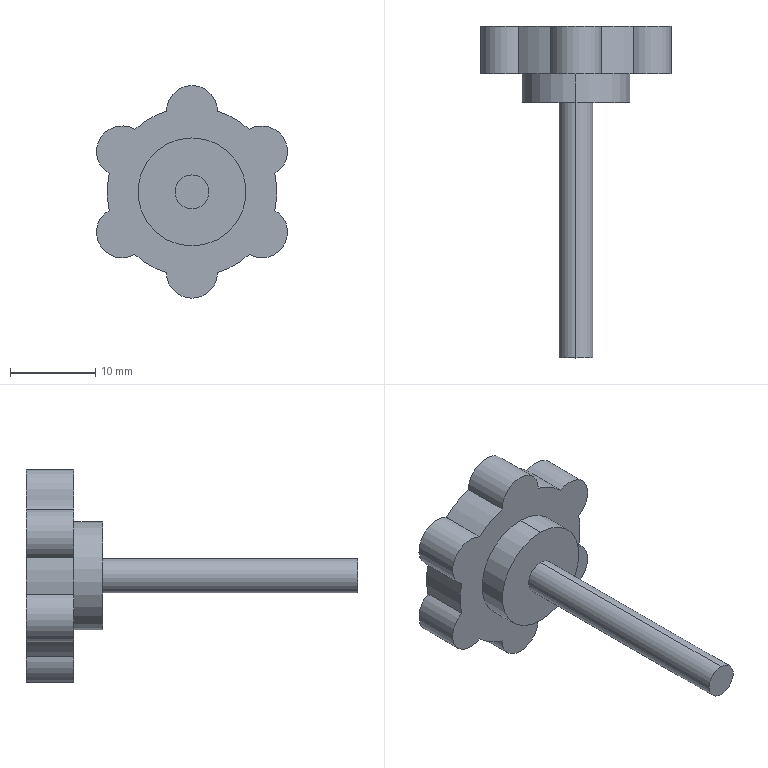Part | SolidWorks | features ICE 2, Extrusion 1 | 1 solid | 34 faces | box 22.455 x 39 x 25 mm | volume 2966 mm3 | cylinder 19 | plane 15 | commonest cylinder face diameters 6 x9 19.922 x6 4 x2 12.7 x2
STEP:
#1=CARTESIAN_POINT('',(0.,-33.4,-2.));
#2=VERTEX_POINT('',#1);
#3=CARTESIAN_POINT('',(0.,-33.4,2.));
#4=VERTEX_POINT('',#3);
#5=CARTESIAN_POINT('',(0.,-33.4,0.));
#6=DIRECTION('',(0.,-1.,0.));
#7=DIRECTION('',(0.,0.,-1.));
#8=AXIS2_PLACEMENT_3D('',#5,#6,#7);
#9=CIRCLE('',#8,2.);
#10=EDGE_CURVE('',#2,#4,#9,.T.);
#11=ORIENTED_EDGE('',*,*,#10,.F.);
#12=CARTESIAN_POINT('',(0.,-3.4,-2.));
#13=VERTEX_POINT('',#12);
#14=CARTESIAN_POINT('',(0.,-33.4,-2.));
#15=DIRECTION('',(0.,1.,0.));
#16=VECTOR('',#15,1000.);
#17=LINE('',#14,#16);
#18=EDGE_CURVE('',#2,#13,#17,.T.);
#19=ORIENTED_EDGE('',*,*,#18,.T.);
#20=CARTESIAN_POINT('',(0.,-3.4,2.));
#21=VERTEX_POINT('',#20);
#22=CARTESIAN_POINT('',(0.,-3.4,0.));
#23=DIRECTION('',(0.,-1.,0.));
#24=DIRECTION('',(0.,0.,-1.));
#25=AXIS2_PLACEMENT_3D('',#22,#23,#24);
#26=CIRCLE('',#25,2.);
#27=EDGE_CURVE('',#13,#21,#26,.T.);
#28=ORIENTED_EDGE('',*,*,#27,.T.);
#29=CARTESIAN_POINT('',(0.,-33.4,2.));
#30=DIRECTION('',(0.,1.,0.));
#31=VECTOR('',#30,1000.);
#32=LINE('',#29,#31);
#33=EDGE_CURVE('',#4,#21,#32,.T.);
#34=ORIENTED_EDGE('',*,*,#33,.F.);
#35=EDGE_LOOP('',(#11,#19,#28,#34));
#36=FACE_OUTER_BOUND('',#35,.T.);
#37=CARTESIAN_POINT('',(0.,-33.4,0.));
#38=DIRECTION('',(0.,1.,0.));
#39=DIRECTION('',(0.,0.,1.));
#40=AXIS2_PLACEMENT_3D('',#37,#38,#39);
#41=CYLINDRICAL_SURFACE('',#40,2.);
#42=ADVANCED_FACE('',(#36),#41,.T.);
#43=CARTESIAN_POINT('',(0.,-3.4,-6.35));
#44=VERTEX_POINT('',#43);
#45=CARTESIAN_POINT('',(0.,-3.4,6.35));
#46=VERTEX_POINT('',#45);
#47=CARTESIAN_POINT('',(0.,-3.4,0.));
#48=DIRECTION('',(0.,-1.,0.));
#49=DIRECTION('',(0.,0.,-1.));
#50=AXIS2_PLACEMENT_3D('',#47,#48,#49);
#51=CIRCLE('',#50,6.35);
#52=EDGE_CURVE('',#44,#46,#51,.T.);
#53=ORIENTED_EDGE('',*,*,#52,.F.);
#54=CARTESIAN_POINT('',(0.,0.,-6.35));
#55=VERTEX_POINT('',#54);
#56=CARTESIAN_POINT('',(0.,-3.4,-6.35));
#57=DIRECTION('',(0.,1.,0.));
#58=VECTOR('',#57,1000.);
#59=LINE('',#56,#58);
#60=EDGE_CURVE('',#44,#55,#59,.T.);
#61=ORIENTED_EDGE('',*,*,#60,.T.);
#62=CARTESIAN_POINT('',(0.,0.,6.35));
#63=VERTEX_POINT('',#62);
#64=CARTESIAN_POINT('',(0.,0.,0.));
#65=DIRECTION('',(0.,-1.,0.));
#66=DIRECTION('',(0.,0.,1.));
#67=AXIS2_PLACEMENT_3D('',#64,#65,#66);
#68=CIRCLE('',#67,6.35);
#69=EDGE_CURVE('',#55,#63,#68,.T.);
#70=ORIENTED_EDGE('',*,*,#69,.T.);
#71=CARTESIAN_POINT('',(0.,-3.4,6.35));
#72=DIRECTION('',(0.,1.,0.));
#73=VECTOR('',#72,1000.);
#74=LINE('',#71,#73);
#75=EDGE_CURVE('',#46,#63,#74,.T.);
#76=ORIENTED_EDGE('',*,*,#75,.F.);
#77=EDGE_LOOP('',(#53,#61,#70,#76));
#78=FACE_OUTER_BOUND('',#77,.T.);
#79=CARTESIAN_POINT('',(0.,-3.4,0.));
#80=DIRECTION('',(0.,1.,0.));
#81=DIRECTION('',(0.,0.,1.));
#82=AXIS2_PLACEMENT_3D('',#79,#80,#81);
#83=CYLINDRICAL_SURFACE('',#82,6.35);
#84=ADVANCED_FACE('',(#78),#83,.T.);
#85=CARTESIAN_POINT('',(8.228,5.6,-7.751));
#86=VERTEX_POINT('',#85);
#87=CARTESIAN_POINT('',(6.728,5.6,-7.349));
#88=VERTEX_POINT('',#87);
#89=CARTESIAN_POINT('',(8.228,5.6,-4.751));
#90=DIRECTION('',(0.,1.,0.));
#91=DIRECTION('',(0.,0.,1.));
#92=AXIS2_PLACEMENT_3D('',#89,#90,#91);
#93=CIRCLE('',#92,3.);
#94=EDGE_CURVE('',#86,#88,#93,.T.);
#95=ORIENTED_EDGE('',*,*,#94,.F.);
#96=CARTESIAN_POINT('',(8.228,0.,-7.751));
#97=VERTEX_POINT('',#96);
#98=CARTESIAN_POINT('',(8.228,5.6,-7.751));
#99=DIRECTION('',(0.,-1.,0.));
#100=VECTOR('',#99,1000.);
#101=LINE('',#98,#100);
#102=EDGE_CURVE('',#86,#97,#101,.T.);
#103=ORIENTED_EDGE('',*,*,#102,.T.);
#104=CARTESIAN_POINT('',(6.728,0.,-7.349));
#105=VERTEX_POINT('',#104);
#106=CARTESIAN_POINT('',(8.228,0.,-4.751));
#107=DIRECTION('',(0.,1.,0.));
#108=DIRECTION('',(0.,0.,1.));
#109=AXIS2_PLACEMENT_3D('',#106,#107,#108);
#110=CIRCLE('',#109,3.);
#111=EDGE_CURVE('',#97,#105,#110,.T.);
#112=ORIENTED_EDGE('',*,*,#111,.T.);
#113=CARTESIAN_POINT('',(6.728,5.6,-7.349));
#114=DIRECTION('',(0.,-1.,0.));
#115=VECTOR('',#114,1000.);
#116=LINE('',#113,#115);
#117=EDGE_CURVE('',#88,#105,#116,.T.);
#118=ORIENTED_EDGE('',*,*,#117,.F.);
#119=EDGE_LOOP('',(#95,#103,#112,#118));
#120=FACE_OUTER_BOUND('',#119,.T.);
#121=CARTESIAN_POINT('',(8.228,5.6,-4.751));
#122=DIRECTION('',(0.,-1.,0.));
#123=DIRECTION('',(0.,0.,-1.));
#124=AXIS2_PLACEMENT_3D('',#121,#122,#123);
#125=CYLINDRICAL_SURFACE('',#124,3.);
#126=ADVANCED_FACE('',(#120),#125,.T.);
#127=CARTESIAN_POINT('',(-8.227,5.6,-7.749));
#128=VERTEX_POINT('',#127);
#129=CARTESIAN_POINT('',(-9.727,5.6,-2.151));
#130=VERTEX_POINT('',#129);
#131=CARTESIAN_POINT('',(-8.227,5.6,-4.749));
#132=DIRECTION('',(0.,1.,0.));
#133=DIRECTION('',(0.,0.,1.));
#134=AXIS2_PLACEMENT_3D('',#131,#132,#133);
#135=CIRCLE('',#134,3.);
#136=EDGE_CURVE('',#128,#130,#135,.T.);
#137=ORIENTED_EDGE('',*,*,#136,.F.);
#138=CARTESIAN_POINT('',(-8.227,0.,-7.749));
#139=VERTEX_POINT('',#138);
#140=CARTESIAN_POINT('',(-8.227,5.6,-7.749));
#141=DIRECTION('',(0.,-1.,0.));
#142=VECTOR('',#141,1000.);
#143=LINE('',#140,#142);
#144=EDGE_CURVE('',#128,#139,#143,.T.);
#145=ORIENTED_EDGE('',*,*,#144,.T.);
#146=CARTESIAN_POINT('',(-9.727,0.,-2.151));
#147=VERTEX_POINT('',#146);
#148=CARTESIAN_POINT('',(-8.227,0.,-4.749));
#149=DIRECTION('',(0.,1.,0.));
#150=DIRECTION('',(0.,0.,1.));
#151=AXIS2_PLACEMENT_3D('',#148,#149,#150);
#152=CIRCLE('',#151,3.);
#153=EDGE_CURVE('',#139,#147,#152,.T.);
#154=ORIENTED_EDGE('',*,*,#153,.T.);
#155=CARTESIAN_POINT('',(-9.727,5.6,-2.151));
#156=DIRECTION('',(0.,-1.,0.));
#157=VECTOR('',#156,1000.);
#158=LINE('',#155,#157);
#159=EDGE_CURVE('',#130,#147,#158,.T.);
#160=ORIENTED_EDGE('',*,*,#159,.F.);
#161=EDGE_LOOP('',(#137,#145,#154,#160));
#162=FACE_OUTER_BOUND('',#161,.T.);
#163=CARTESIAN_POINT('',(-8.227,5.6,-4.749));
#164=DIRECTION('',(0.,-1.,0.));
#165=DIRECTION('',(0.,0.,-1.));
#166=AXIS2_PLACEMENT_3D('',#163,#164,#165);
#167=CYLINDRICAL_SURFACE('',#166,3.);
#168=ADVANCED_FACE('',(#162),#167,.T.);
#169=CARTESIAN_POINT('',(0.,5.6,-12.5));
#170=VERTEX_POINT('',#169);
#171=CARTESIAN_POINT('',(-3.,5.6,-9.5));
#172=VERTEX_POINT('',#171);
#173=CARTESIAN_POINT('',(0.,5.6,-9.5));
#174=DIRECTION('',(0.,1.,0.));
#175=DIRECTION('',(0.,0.,1.));
#176=AXIS2_PLACEMENT_3D('',#173,#174,#175);
#177=CIRCLE('',#176,3.);
#178=EDGE_CURVE('',#170,#172,#177,.T.);
#179=ORIENTED_EDGE('',*,*,#178,.F.);
#180=CARTESIAN_POINT('',(0.,0.,-12.5));
#181=VERTEX_POINT('',#180);
#182=CARTESIAN_POINT('',(0.,5.6,-12.5));
#183=DIRECTION('',(0.,-1.,0.));
#184=VECTOR('',#183,1000.);
#185=LINE('',#182,#184);
#186=EDGE_CURVE('',#170,#181,#185,.T.);
#187=ORIENTED_EDGE('',*,*,#186,.T.);
#188=CARTESIAN_POINT('',(-3.,0.,-9.5));
#189=VERTEX_POINT('',#188);
#190=CARTESIAN_POINT('',(0.,0.,-9.5));
#191=DIRECTION('',(0.,1.,0.));
#192=DIRECTION('',(0.,0.,1.));
#193=AXIS2_PLACEMENT_3D('',#190,#191,#192);
#194=CIRCLE('',#193,3.);
#195=EDGE_CURVE('',#181,#189,#194,.T.);
#196=ORIENTED_EDGE('',*,*,#195,.T.);
#197=CARTESIAN_POINT('',(-3.,5.6,-9.5));
#198=DIRECTION('',(0.,-1.,0.));
#199=VECTOR('',#198,1000.);
#200=LINE('',#197,#199);
#201=EDGE_CURVE('',#172,#189,#200,.T.);
#202=ORIENTED_EDGE('',*,*,#201,.F.);
#203=EDGE_LOOP('',(#179,#187,#196,#202));
#204=FACE_OUTER_BOUND('',#203,.T.);
#205=CARTESIAN_POINT('',(0.,5.6,-9.5));
#206=DIRECTION('',(0.,-1.,0.));
#207=DIRECTION('',(0.,0.,-1.));
#208=AXIS2_PLACEMENT_3D('',#205,#206,#207);
#209=CYLINDRICAL_SURFACE('',#208,3.);
#210=ADVANCED_FACE('',(#204),#209,.T.);
#211=ORIENTED_EDGE('',*,*,#186,.F.);
#212=CARTESIAN_POINT('',(3.,5.6,-9.5));
#213=VERTEX_POINT('',#212);
#214=CARTESIAN_POINT('',(0.,5.6,-9.5));
#215=DIRECTION('',(0.,1.,0.));
#216=DIRECTION('',(0.,0.,1.));
#217=AXIS2_PLACEMENT_3D('',#214,#215,#216);
#218=CIRCLE('',#217,3.);
#219=EDGE_CURVE('',#213,#170,#218,.T.);
#220=ORIENTED_EDGE('',*,*,#219,.F.);
#221=CARTESIAN_POINT('',(3.,0.,-9.5));
#222=VERTEX_POINT('',#221);
#223=CARTESIAN_POINT('',(3.,5.6,-9.5));
#224=DIRECTION('',(0.,-1.,0.));
#225=VECTOR('',#224,1000.);
#226=LINE('',#223,#225);
#227=EDGE_CURVE('',#213,#222,#226,.T.);
#228=ORIENTED_EDGE('',*,*,#227,.T.);
#229=CARTESIAN_POINT('',(0.,0.,-9.5));
#230=DIRECTION('',(0.,1.,0.));
#231=DIRECTION('',(0.,0.,1.));
#232=AXIS2_PLACEMENT_3D('',#229,#230,#231);
#233=CIRCLE('',#232,3.);
#234=EDGE_CURVE('',#222,#181,#233,.T.);
#235=ORIENTED_EDGE('',*,*,#234,.T.);
#236=EDGE_LOOP('',(#211,#220,#228,#235));
#237=FACE_OUTER_BOUND('',#236,.T.);
#238=CARTESIAN_POINT('',(0.,5.6,-9.5));
#239=DIRECTION('',(0.,-1.,0.));
#240=DIRECTION('',(0.,0.,-1.));
#241=AXIS2_PLACEMENT_3D('',#238,#239,#240);
#242=CYLINDRICAL_SURFACE('',#241,3.);
#243=ADVANCED_FACE('',(#237),#242,.T.);
#244=CARTESIAN_POINT('',(-3.,0.,-9.499));
#245=VERTEX_POINT('',#244);
#246=CARTESIAN_POINT('',(-3.,0.,-9.499));
#247=DIRECTION('',(0.,0.,1.));
#248=VECTOR('',#247,1000.);
#249=LINE('',#246,#248);
#250=EDGE_CURVE('',#189,#245,#249,.T.);
#251=ORIENTED_EDGE('',*,*,#250,.T.);
#252=CARTESIAN_POINT('',(-3.,5.6,-9.499));
#253=VERTEX_POINT('',#252);
#254=CARTESIAN_POINT('',(-3.,5.6,-9.499));
#255=DIRECTION('',(0.,-1.,0.));
#256=VECTOR('',#255,1000.);
#257=LINE('',#254,#256);
#258=EDGE_CURVE('',#253,#245,#257,.T.);
#259=ORIENTED_EDGE('',*,*,#258,.F.);
#260=CARTESIAN_POINT('',(-3.,5.6,-9.499));
#261=DIRECTION('',(0.,0.,1.));
#262=VECTOR('',#261,1000.);
#263=LINE('',#260,#262);
#264=EDGE_CURVE('',#172,#253,#263,.T.);
#265=ORIENTED_EDGE('',*,*,#264,.F.);
#266=ORIENTED_EDGE('',*,*,#201,.T.);
#267=EDGE_LOOP('',(#251,#259,#265,#266));
#268=FACE_OUTER_BOUND('',#267,.T.);
#269=CARTESIAN_POINT('',(-3.,5.6,-9.499));
#270=DIRECTION('',(1.,0.,0.));
#271=DIRECTION('',(0.,0.,-1.));
#272=AXIS2_PLACEMENT_3D('',#269,#270,#271);
#273=PLANE('',#272);
#274=ADVANCED_FACE('',(#268),#273,.F.);
#275=CARTESIAN_POINT('',(-6.726,0.,-7.347));
#276=VERTEX_POINT('',#275);
#277=CARTESIAN_POINT('',(0.0015,0.,-0.000866));
#278=DIRECTION('',(0.,1.,0.));
#279=DIRECTION('',(0.,0.,1.));
#280=AXIS2_PLACEMENT_3D('',#277,#278,#279);
#281=CIRCLE('',#280,9.961);
#282=EDGE_CURVE('',#245,#276,#281,.T.);
#283=ORIENTED_EDGE('',*,*,#282,.T.);
#284=CARTESIAN_POINT('',(-6.726,5.6,-7.347));
#285=VERTEX_POINT('',#284);
#286=CARTESIAN_POINT('',(-6.726,5.6,-7.347));
#287=DIRECTION('',(0.,-1.,0.));
#288=VECTOR('',#287,1000.);
#289=LINE('',#286,#288);
#290=EDGE_CURVE('',#285,#276,#289,.T.);
#291=ORIENTED_EDGE('',*,*,#290,.F.);
#292=CARTESIAN_POINT('',(0.0015,5.6,-0.000866));
#293=DIRECTION('',(0.,1.,0.));
#294=DIRECTION('',(0.,0.,1.));
#295=AXIS2_PLACEMENT_3D('',#292,#293,#294);
#296=CIRCLE('',#295,9.961);
#297=EDGE_CURVE('',#253,#285,#296,.T.);
#298=ORIENTED_EDGE('',*,*,#297,.F.);
#299=ORIENTED_EDGE('',*,*,#258,.T.);
#300=EDGE_LOOP('',(#283,#291,#298,#299));
#301=FACE_OUTER_BOUND('',#300,.T.);
#302=CARTESIAN_POINT('',(0.0015,5.6,-0.000866));
#303=DIRECTION('',(0.,-1.,0.));
#304=DIRECTION('',(0.,0.,-1.));
#305=AXIS2_PLACEMENT_3D('',#302,#303,#304);
#306=CYLINDRICAL_SURFACE('',#305,9.961);
#307=ADVANCED_FACE('',(#301),#306,.T.);
#308=CARTESIAN_POINT('',(-6.727,0.,-7.347));
#309=VERTEX_POINT('',#308);
#310=CARTESIAN_POINT('',(-6.726,0.,-7.347));
#311=DIRECTION('',(-0.866,0.,-0.5));
#312=VECTOR('',#311,1000.);
#313=LINE('',#310,#312);
#314=EDGE_CURVE('',#276,#309,#313,.T.);
#315=ORIENTED_EDGE('',*,*,#314,.T.);
#316=CARTESIAN_POINT('',(-6.727,5.6,-7.347));
#317=VERTEX_POINT('',#316);
#318=CARTESIAN_POINT('',(-6.727,5.6,-7.347));
#319=DIRECTION('',(0.,-1.,0.));
#320=VECTOR('',#319,1000.);
#321=LINE('',#318,#320);
#322=EDGE_CURVE('',#317,#309,#321,.T.);
#323=ORIENTED_EDGE('',*,*,#322,.F.);
#324=CARTESIAN_POINT('',(-6.726,5.6,-7.347));
#325=DIRECTION('',(-0.866,0.,-0.5));
#326=VECTOR('',#325,1000.);
#327=LINE('',#324,#326);
#328=EDGE_CURVE('',#285,#317,#327,.T.);
#329=ORIENTED_EDGE('',*,*,#328,.F.);
#330=ORIENTED_EDGE('',*,*,#290,.T.);
#331=EDGE_LOOP('',(#315,#323,#329,#330));
#332=FACE_OUTER_BOUND('',#331,.T.);
#333=CARTESIAN_POINT('',(-6.726,5.6,-7.347));
#334=DIRECTION('',(-0.5,0.,0.866));
#335=DIRECTION('',(0.866,0.,0.5));
#336=AXIS2_PLACEMENT_3D('',#333,#334,#335);
#337=PLANE('',#336);
#338=ADVANCED_FACE('',(#332),#337,.F.);
#339=ORIENTED_EDGE('',*,*,#144,.F.);
#340=CARTESIAN_POINT('',(-8.227,5.6,-4.749));
#341=DIRECTION('',(0.,1.,0.));
#342=DIRECTION('',(0.,0.,1.));
#343=AXIS2_PLACEMENT_3D('',#340,#341,#342);
#344=CIRCLE('',#343,3.);
#345=EDGE_CURVE('',#317,#128,#344,.T.);
#346=ORIENTED_EDGE('',*,*,#345,.F.);
#347=ORIENTED_EDGE('',*,*,#322,.T.);
#348=CARTESIAN_POINT('',(-8.227,0.,-4.749));
#349=DIRECTION('',(0.,1.,0.));
#350=DIRECTION('',(0.,0.,1.));
#351=AXIS2_PLACEMENT_3D('',#348,#349,#350);
#352=CIRCLE('',#351,3.);
#353=EDGE_CURVE('',#309,#139,#352,.T.);
#354=ORIENTED_EDGE('',*,*,#353,.T.);
#355=EDGE_LOOP('',(#339,#346,#347,#354));
#356=FACE_OUTER_BOUND('',#355,.T.);
#357=CARTESIAN_POINT('',(-8.227,5.6,-4.749));
#358=DIRECTION('',(0.,-1.,0.));
#359=DIRECTION('',(0.,0.,-1.));
#360=AXIS2_PLACEMENT_3D('',#357,#358,#359);
#361=CYLINDRICAL_SURFACE('',#360,3.);
#362=ADVANCED_FACE('',(#356),#361,.T.);
#363=CARTESIAN_POINT('',(-9.725,0.,-2.15));
#364=VERTEX_POINT('',#363);
#365=CARTESIAN_POINT('',(-9.725,0.,-2.15));
#366=DIRECTION('',(0.866,0.,0.5));
#367=VECTOR('',#366,1000.);
#368=LINE('',#365,#367);
#369=EDGE_CURVE('',#147,#364,#368,.T.);
#370=ORIENTED_EDGE('',*,*,#369,.T.);
#371=CARTESIAN_POINT('',(-9.725,5.6,-2.15));
#372=VERTEX_POINT('',#371);
#373=CARTESIAN_POINT('',(-9.725,5.6,-2.15));
#374=DIRECTION('',(0.,-1.,0.));
#375=VECTOR('',#374,1000.);
#376=LINE('',#373,#375);
#377=EDGE_CURVE('',#372,#364,#376,.T.);
#378=ORIENTED_EDGE('',*,*,#377,.F.);
#379=CARTESIAN_POINT('',(-9.725,5.6,-2.15));
#380=DIRECTION('',(0.866,0.,0.5));
#381=VECTOR('',#380,1000.);
#382=LINE('',#379,#381);
#383=EDGE_CURVE('',#130,#372,#382,.T.);
#384=ORIENTED_EDGE('',*,*,#383,.F.);
#385=ORIENTED_EDGE('',*,*,#159,.T.);
#386=EDGE_LOOP('',(#370,#378,#384,#385));
#387=FACE_OUTER_BOUND('',#386,.T.);
#388=CARTESIAN_POINT('',(-9.725,5.6,-2.15));
#389=DIRECTION('',(0.5,0.,-0.866));
#390=DIRECTION('',(-0.866,0.,-0.5));
#391=AXIS2_PLACEMENT_3D('',#388,#389,#390);
#392=PLANE('',#391);
#393=ADVANCED_FACE('',(#387),#392,.F.);
#394=CARTESIAN_POINT('',(-9.724,0.,2.152));
#395=VERTEX_POINT('',#394);
#396=CARTESIAN_POINT('',(0.0015,0.,-0.000866));
#397=DIRECTION('',(0.,1.,0.));
#398=DIRECTION('',(0.,0.,1.));
#399=AXIS2_PLACEMENT_3D('',#396,#397,#398);
#400=CIRCLE('',#399,9.961);
#401=EDGE_CURVE('',#364,#395,#400,.T.);
#402=ORIENTED_EDGE('',*,*,#401,.T.);
#403=CARTESIAN_POINT('',(-9.724,5.6,2.152));
#404=VERTEX_POINT('',#403);
#405=CARTESIAN_POINT('',(-9.724,5.6,2.152));
#406=DIRECTION('',(0.,-1.,0.));
#407=VECTOR('',#406,1000.);
#408=LINE('',#405,#407);
#409=EDGE_CURVE('',#404,#395,#408,.T.);
#410=ORIENTED_EDGE('',*,*,#409,.F.);
#411=CARTESIAN_POINT('',(0.0015,5.6,-0.000866));
#412=DIRECTION('',(0.,1.,0.));
#413=DIRECTION('',(0.,0.,1.));
#414=AXIS2_PLACEMENT_3D('',#411,#412,#413);
#415=CIRCLE('',#414,9.961);
#416=EDGE_CURVE('',#372,#404,#415,.T.);
#417=ORIENTED_EDGE('',*,*,#416,.F.);
#418=ORIENTED_EDGE('',*,*,#377,.T.);
#419=EDGE_LOOP('',(#402,#410,#417,#418));
#420=FACE_OUTER_BOUND('',#419,.T.);
#421=CARTESIAN_POINT('',(0.0015,5.6,-0.000866));
#422=DIRECTION('',(0.,-1.,0.));
#423=DIRECTION('',(0.,0.,-1.));
#424=AXIS2_PLACEMENT_3D('',#421,#422,#423);
#425=CYLINDRICAL_SURFACE('',#424,9.961);
#426=ADVANCED_FACE('',(#420),#425,.T.);
#427=CARTESIAN_POINT('',(-9.726,0.,2.153));
#428=VERTEX_POINT('',#427);
#429=CARTESIAN_POINT('',(-9.724,0.,2.152));
#430=DIRECTION('',(-0.866,0.,0.5));
#431=VECTOR('',#430,1000.);
#432=LINE('',#429,#431);
#433=EDGE_CURVE('',#395,#428,#432,.T.);
#434=ORIENTED_EDGE('',*,*,#433,.T.);
#435=CARTESIAN_POINT('',(-9.726,5.6,2.153));
#436=VERTEX_POINT('',#435);
#437=CARTESIAN_POINT('',(-9.726,5.6,2.153));
#438=DIRECTION('',(0.,-1.,0.));
#439=VECTOR('',#438,1000.);
#440=LINE('',#437,#439);
#441=EDGE_CURVE('',#436,#428,#440,.T.);
#442=ORIENTED_EDGE('',*,*,#441,.F.);
#443=CARTESIAN_POINT('',(-9.724,5.6,2.152));
#444=DIRECTION('',(-0.866,0.,0.5));
#445=VECTOR('',#444,1000.);
#446=LINE('',#443,#445);
#447=EDGE_CURVE('',#404,#436,#446,.T.);
#448=ORIENTED_EDGE('',*,*,#447,.F.);
#449=ORIENTED_EDGE('',*,*,#409,.T.);
#450=EDGE_LOOP('',(#434,#442,#448,#449));
#451=FACE_OUTER_BOUND('',#450,.T.);
#452=CARTESIAN_POINT('',(-9.724,5.6,2.152));
#453=DIRECTION('',(0.5,0.,0.866));
#454=DIRECTION('',(0.866,0.,-0.5));
#455=AXIS2_PLACEMENT_3D('',#452,#453,#454);
#456=PLANE('',#455);
#457=ADVANCED_FACE('',(#451),#456,.F.);
#458=CARTESIAN_POINT('',(-6.726,0.,7.349));
#459=VERTEX_POINT('',#458);
#460=CARTESIAN_POINT('',(-8.226,0.,4.751));
#461=DIRECTION('',(0.,1.,0.));
#462=DIRECTION('',(0.,0.,1.));
#463=AXIS2_PLACEMENT_3D('',#460,#461,#462);
#464=CIRCLE('',#463,3.);
#465=EDGE_CURVE('',#428,#459,#464,.T.);
#466=ORIENTED_EDGE('',*,*,#465,.T.);
#467=CARTESIAN_POINT('',(-6.726,5.6,7.349));
#468=VERTEX_POINT('',#467);
#469=CARTESIAN_POINT('',(-6.726,5.6,7.349));
#470=DIRECTION('',(0.,-1.,0.));
#471=VECTOR('',#470,1000.);
#472=LINE('',#469,#471);
#473=EDGE_CURVE('',#468,#459,#472,.T.);
#474=ORIENTED_EDGE('',*,*,#473,.F.);
#475=CARTESIAN_POINT('',(-8.226,5.6,4.751));
#476=DIRECTION('',(0.,1.,0.));
#477=DIRECTION('',(0.,0.,1.));
#478=AXIS2_PLACEMENT_3D('',#475,#476,#477);
#479=CIRCLE('',#478,3.);
#480=EDGE_CURVE('',#436,#468,#479,.T.);
#481=ORIENTED_EDGE('',*,*,#480,.F.);
#482=ORIENTED_EDGE('',*,*,#441,.T.);
#483=EDGE_LOOP('',(#466,#474,#481,#482));
#484=FACE_OUTER_BOUND('',#483,.T.);
#485=CARTESIAN_POINT('',(-8.226,5.6,4.751));
#486=DIRECTION('',(0.,-1.,0.));
#487=DIRECTION('',(0.,0.,-1.));
#488=AXIS2_PLACEMENT_3D('',#485,#486,#487);
#489=CYLINDRICAL_SURFACE('',#488,3.);
#490=ADVANCED_FACE('',(#484),#489,.T.);
#491=CARTESIAN_POINT('',(-6.723,0.,7.348));
#492=VERTEX_POINT('',#491);
#493=CARTESIAN_POINT('',(-6.723,0.,7.348));
#494=DIRECTION('',(0.866,0.,-0.5));
#495=VECTOR('',#494,1000.);
#496=LINE('',#493,#495);
#497=EDGE_CURVE('',#459,#492,#496,.T.);
#498=ORIENTED_EDGE('',*,*,#497,.T.);
#499=CARTESIAN_POINT('',(-6.723,5.6,7.348));
#500=VERTEX_POINT('',#499);
#501=CARTESIAN_POINT('',(-6.723,5.6,7.348));
#502=DIRECTION('',(0.,-1.,0.));
#503=VECTOR('',#502,1000.);
#504=LINE('',#501,#503);
#505=EDGE_CURVE('',#500,#492,#504,.T.);
#506=ORIENTED_EDGE('',*,*,#505,.F.);
#507=CARTESIAN_POINT('',(-6.723,5.6,7.348));
#508=DIRECTION('',(0.866,0.,-0.5));
#509=VECTOR('',#508,1000.);
#510=LINE('',#507,#509);
#511=EDGE_CURVE('',#468,#500,#510,.T.);
#512=ORIENTED_EDGE('',*,*,#511,.F.);
#513=ORIENTED_EDGE('',*,*,#473,.T.);
#514=EDGE_LOOP('',(#498,#506,#512,#513));
#515=FACE_OUTER_BOUND('',#514,.T.);
#516=CARTESIAN_POINT('',(-6.723,5.6,7.348));
#517=DIRECTION('',(-0.5,0.,-0.866));
#518=DIRECTION('',(-0.866,0.,0.5));
#519=AXIS2_PLACEMENT_3D('',#516,#517,#518);
#520=PLANE('',#519);
#521=ADVANCED_FACE('',(#515),#520,.F.);
#522=CARTESIAN_POINT('',(-2.998,0.,9.498));
#523=VERTEX_POINT('',#522);
#524=CARTESIAN_POINT('',(0.0015,0.,-0.000866));
#525=DIRECTION('',(0.,1.,0.));
#526=DIRECTION('',(0.,0.,1.));
#527=AXIS2_PLACEMENT_3D('',#524,#525,#526);
#528=CIRCLE('',#527,9.961);
#529=EDGE_CURVE('',#492,#523,#528,.T.);
#530=ORIENTED_EDGE('',*,*,#529,.T.);
#531=CARTESIAN_POINT('',(-2.998,5.6,9.498));
#532=VERTEX_POINT('',#531);
#533=CARTESIAN_POINT('',(-2.998,5.6,9.498));
#534=DIRECTION('',(0.,-1.,0.));
#535=VECTOR('',#534,1000.);
#536=LINE('',#533,#535);
#537=EDGE_CURVE('',#532,#523,#536,.T.);
#538=ORIENTED_EDGE('',*,*,#537,.F.);
#539=CARTESIAN_POINT('',(0.0015,5.6,-0.000866));
#540=DIRECTION('',(0.,1.,0.));
#541=DIRECTION('',(0.,0.,1.));
#542=AXIS2_PLACEMENT_3D('',#539,#540,#541);
#543=CIRCLE('',#542,9.961);
#544=EDGE_CURVE('',#500,#532,#543,.T.);
#545=ORIENTED_EDGE('',*,*,#544,.F.);
#546=ORIENTED_EDGE('',*,*,#505,.T.);
#547=EDGE_LOOP('',(#530,#538,#545,#546));
#548=FACE_OUTER_BOUND('',#547,.T.);
#549=CARTESIAN_POINT('',(0.0015,5.6,-0.000866));
#550=DIRECTION('',(0.,-1.,0.));
#551=DIRECTION('',(0.,0.,-1.));
#552=AXIS2_PLACEMENT_3D('',#549,#550,#551);
#553=CYLINDRICAL_SURFACE('',#552,9.961);
#554=ADVANCED_FACE('',(#548),#553,.T.);
#555=CARTESIAN_POINT('',(-2.998,0.,9.5));
#556=VERTEX_POINT('',#555);
#557=CARTESIAN_POINT('',(-2.998,0.,9.498));
#558=DIRECTION('',(0.,0.,1.));
#559=VECTOR('',#558,1000.);
#560=LINE('',#557,#559);
#561=EDGE_CURVE('',#523,#556,#560,.T.);
#562=ORIENTED_EDGE('',*,*,#561,.T.);
#563=CARTESIAN_POINT('',(-2.998,5.6,9.5));
#564=VERTEX_POINT('',#563);
#565=CARTESIAN_POINT('',(-2.998,5.6,9.5));
#566=DIRECTION('',(0.,-1.,0.));
#567=VECTOR('',#566,1000.);
#568=LINE('',#565,#567);
#569=EDGE_CURVE('',#564,#556,#568,.T.);
#570=ORIENTED_EDGE('',*,*,#569,.F.);
#571=CARTESIAN_POINT('',(-2.998,5.6,9.498));
#572=DIRECTION('',(0.,0.,1.));
#573=VECTOR('',#572,1000.);
#574=LINE('',#571,#573);
#575=EDGE_CURVE('',#532,#564,#574,.T.);
#576=ORIENTED_EDGE('',*,*,#575,.F.);
#577=ORIENTED_EDGE('',*,*,#537,.T.);
#578=EDGE_LOOP('',(#562,#570,#576,#577));
#579=FACE_OUTER_BOUND('',#578,.T.);
#580=CARTESIAN_POINT('',(-2.998,5.6,9.498));
#581=DIRECTION('',(1.,0.,0.));
#582=DIRECTION('',(0.,0.,-1.));
#583=AXIS2_PLACEMENT_3D('',#580,#581,#582);
#584=PLANE('',#583);
#585=ADVANCED_FACE('',(#579),#584,.F.);
#586=CARTESIAN_POINT('',(3.002,0.,9.5));
#587=VERTEX_POINT('',#586);
#588=CARTESIAN_POINT('',(0.002,0.,9.5));
#589=DIRECTION('',(0.,1.,0.));
#590=DIRECTION('',(0.,0.,1.));
#591=AXIS2_PLACEMENT_3D('',#588,#589,#590);
#592=CIRCLE('',#591,3.);
#593=EDGE_CURVE('',#556,#587,#592,.T.);
#594=ORIENTED_EDGE('',*,*,#593,.T.);
#595=CARTESIAN_POINT('',(3.002,5.6,9.5));
#596=VERTEX_POINT('',#595);
#597=CARTESIAN_POINT('',(3.002,5.6,9.5));
#598=DIRECTION('',(0.,-1.,0.));
#599=VECTOR('',#598,1000.);
#600=LINE('',#597,#599);
#601=EDGE_CURVE('',#596,#587,#600,.T.);
#602=ORIENTED_EDGE('',*,*,#601,.F.);
#603=CARTESIAN_POINT('',(0.002,5.6,9.5));
#604=DIRECTION('',(0.,1.,0.));
#605=DIRECTION('',(0.,0.,1.));
#606=AXIS2_PLACEMENT_3D('',#603,#604,#605);
#607=CIRCLE('',#606,3.);
#608=EDGE_CURVE('',#564,#596,#607,.T.);
#609=ORIENTED_EDGE('',*,*,#608,.F.);
#610=ORIENTED_EDGE('',*,*,#569,.T.);
#611=EDGE_LOOP('',(#594,#602,#609,#610));
#612=FACE_OUTER_BOUND('',#611,.T.);
#613=CARTESIAN_POINT('',(0.002,5.6,9.5));
#614=DIRECTION('',(0.,-1.,0.));
#615=DIRECTION('',(0.,0.,-1.));
#616=AXIS2_PLACEMENT_3D('',#613,#614,#615);
#617=CYLINDRICAL_SURFACE('',#616,3.);
#618=ADVANCED_FACE('',(#612),#617,.T.);
#619=CARTESIAN_POINT('',(3.002,0.,9.498));
#620=VERTEX_POINT('',#619);
#621=CARTESIAN_POINT('',(3.002,0.,9.498));
#622=DIRECTION('',(0.,0.,-1.));
#623=VECTOR('',#622,1000.);
#624=LINE('',#621,#623);
#625=EDGE_CURVE('',#587,#620,#624,.T.);
#626=ORIENTED_EDGE('',*,*,#625,.T.);
#627=CARTESIAN_POINT('',(3.002,5.6,9.498));
#628=VERTEX_POINT('',#627);
#629=CARTESIAN_POINT('',(3.002,5.6,9.498));
#630=DIRECTION('',(0.,-1.,0.));
#631=VECTOR('',#630,1000.);
#632=LINE('',#629,#631);
#633=EDGE_CURVE('',#628,#620,#632,.T.);
#634=ORIENTED_EDGE('',*,*,#633,.F.);
#635=CARTESIAN_POINT('',(3.002,5.6,9.498));
#636=DIRECTION('',(0.,0.,-1.));
#637=VECTOR('',#636,1000.);
#638=LINE('',#635,#637);
#639=EDGE_CURVE('',#596,#628,#638,.T.);
#640=ORIENTED_EDGE('',*,*,#639,.F.);
#641=ORIENTED_EDGE('',*,*,#601,.T.);
#642=EDGE_LOOP('',(#626,#634,#640,#641));
#643=FACE_OUTER_BOUND('',#642,.T.);
#644=CARTESIAN_POINT('',(3.002,5.6,9.498));
#645=DIRECTION('',(-1.,0.,0.));
#646=DIRECTION('',(0.,0.,1.));
#647=AXIS2_PLACEMENT_3D('',#644,#645,#646);
#648=PLANE('',#647);
#649=ADVANCED_FACE('',(#643),#648,.F.);
#650=CARTESIAN_POINT('',(6.728,0.,7.347));
#651=VERTEX_POINT('',#650);
#652=CARTESIAN_POINT('',(0.0015,0.,-0.000866));
#653=DIRECTION('',(0.,1.,0.));
#654=DIRECTION('',(0.,0.,1.));
#655=AXIS2_PLACEMENT_3D('',#652,#653,#654);
#656=CIRCLE('',#655,9.961);
#657=EDGE_CURVE('',#620,#651,#656,.T.);
#658=ORIENTED_EDGE('',*,*,#657,.T.);
#659=CARTESIAN_POINT('',(6.728,5.6,7.347));
#660=VERTEX_POINT('',#659);
#661=CARTESIAN_POINT('',(6.728,5.6,7.347));
#662=DIRECTION('',(0.,-1.,0.));
#663=VECTOR('',#662,1000.);
#664=LINE('',#661,#663);
#665=EDGE_CURVE('',#660,#651,#664,.T.);
#666=ORIENTED_EDGE('',*,*,#665,.F.);
#667=CARTESIAN_POINT('',(0.0015,5.6,-0.000866));
#668=DIRECTION('',(0.,1.,0.));
#669=DIRECTION('',(0.,0.,1.));
#670=AXIS2_PLACEMENT_3D('',#667,#668,#669);
#671=CIRCLE('',#670,9.961);
#672=EDGE_CURVE('',#628,#660,#671,.T.);
#673=ORIENTED_EDGE('',*,*,#672,.F.);
#674=ORIENTED_EDGE('',*,*,#633,.T.);
#675=EDGE_LOOP('',(#658,#666,#673,#674));
#676=FACE_OUTER_BOUND('',#675,.T.);
#677=CARTESIAN_POINT('',(0.0015,5.6,-0.000866));
#678=DIRECTION('',(0.,-1.,0.));
#679=DIRECTION('',(0.,0.,-1.));
#680=AXIS2_PLACEMENT_3D('',#677,#678,#679);
#681=CYLINDRICAL_SURFACE('',#680,9.961);
#682=ADVANCED_FACE('',(#676),#681,.T.);
#683=CARTESIAN_POINT('',(6.729,0.,7.347));
#684=VERTEX_POINT('',#683);
#685=CARTESIAN_POINT('',(6.728,0.,7.347));
#686=DIRECTION('',(0.866,0.,0.5));
#687=VECTOR('',#686,1000.);
#688=LINE('',#685,#687);
#689=EDGE_CURVE('',#651,#684,#688,.T.);
#690=ORIENTED_EDGE('',*,*,#689,.T.);
#691=CARTESIAN_POINT('',(6.729,5.6,7.347));
#692=VERTEX_POINT('',#691);
#693=CARTESIAN_POINT('',(6.729,5.6,7.347));
#694=DIRECTION('',(0.,-1.,0.));
#695=VECTOR('',#694,1000.);
#696=LINE('',#693,#695);
#697=EDGE_CURVE('',#692,#684,#696,.T.);
#698=ORIENTED_EDGE('',*,*,#697,.F.);
#699=CARTESIAN_POINT('',(6.728,5.6,7.347));
#700=DIRECTION('',(0.866,0.,0.5));
#701=VECTOR('',#700,1000.);
#702=LINE('',#699,#701);
#703=EDGE_CURVE('',#660,#692,#702,.T.);
#704=ORIENTED_EDGE('',*,*,#703,.F.);
#705=ORIENTED_EDGE('',*,*,#665,.T.);
#706=EDGE_LOOP('',(#690,#698,#704,#705));
#707=FACE_OUTER_BOUND('',#706,.T.);
#708=CARTESIAN_POINT('',(6.728,5.6,7.347));
#709=DIRECTION('',(0.5,0.,-0.866));
#710=DIRECTION('',(-0.866,0.,-0.5));
#711=AXIS2_PLACEMENT_3D('',#708,#709,#710);
#712=PLANE('',#711);
#713=ADVANCED_FACE('',(#707),#712,.F.);
#714=CARTESIAN_POINT('',(9.729,0.,2.151));
#715=VERTEX_POINT('',#714);
#716=CARTESIAN_POINT('',(8.229,0.,4.749));
#717=DIRECTION('',(0.,1.,0.));
#718=DIRECTION('',(0.,0.,1.));
#719=AXIS2_PLACEMENT_3D('',#716,#717,#718);
#720=CIRCLE('',#719,3.);
#721=EDGE_CURVE('',#684,#715,#720,.T.);
#722=ORIENTED_EDGE('',*,*,#721,.T.);
#723=CARTESIAN_POINT('',(9.729,5.6,2.151));
#724=VERTEX_POINT('',#723);
#725=CARTESIAN_POINT('',(9.729,5.6,2.151));
#726=DIRECTION('',(0.,-1.,0.));
#727=VECTOR('',#726,1000.);
#728=LINE('',#725,#727);
#729=EDGE_CURVE('',#724,#715,#728,.T.);
#730=ORIENTED_EDGE('',*,*,#729,.F.);
#731=CARTESIAN_POINT('',(8.229,5.6,4.749));
#732=DIRECTION('',(0.,1.,0.));
#733=DIRECTION('',(0.,0.,1.));
#734=AXIS2_PLACEMENT_3D('',#731,#732,#733);
#735=CIRCLE('',#734,3.);
#736=EDGE_CURVE('',#692,#724,#735,.T.);
#737=ORIENTED_EDGE('',*,*,#736,.F.);
#738=ORIENTED_EDGE('',*,*,#697,.T.);
#739=EDGE_LOOP('',(#722,#730,#737,#738));
#740=FACE_OUTER_BOUND('',#739,.T.);
#741=CARTESIAN_POINT('',(8.229,5.6,4.749));
#742=DIRECTION('',(0.,-1.,0.));
#743=DIRECTION('',(0.,0.,-1.));
#744=AXIS2_PLACEMENT_3D('',#741,#742,#743);
#745=CYLINDRICAL_SURFACE('',#744,3.);
#746=ADVANCED_FACE('',(#740),#745,.T.);
#747=CARTESIAN_POINT('',(9.728,0.,2.15));
#748=VERTEX_POINT('',#747);
#749=CARTESIAN_POINT('',(9.728,0.,2.15));
#750=DIRECTION('',(-0.866,0.,-0.5));
#751=VECTOR('',#750,1000.);
#752=LINE('',#749,#751);
#753=EDGE_CURVE('',#715,#748,#752,.T.);
#754=ORIENTED_EDGE('',*,*,#753,.T.);
#755=CARTESIAN_POINT('',(9.728,5.6,2.15));
#756=VERTEX_POINT('',#755);
#757=CARTESIAN_POINT('',(9.728,5.6,2.15));
#758=DIRECTION('',(0.,-1.,0.));
#759=VECTOR('',#758,1000.);
#760=LINE('',#757,#759);
#761=EDGE_CURVE('',#756,#748,#760,.T.);
#762=ORIENTED_EDGE('',*,*,#761,.F.);
#763=CARTESIAN_POINT('',(9.728,5.6,2.15));
#764=DIRECTION('',(-0.866,0.,-0.5));
#765=VECTOR('',#764,1000.);
#766=LINE('',#763,#765);
#767=EDGE_CURVE('',#724,#756,#766,.T.);
#768=ORIENTED_EDGE('',*,*,#767,.F.);
#769=ORIENTED_EDGE('',*,*,#729,.T.);
#770=EDGE_LOOP('',(#754,#762,#768,#769));
#771=FACE_OUTER_BOUND('',#770,.T.);
#772=CARTESIAN_POINT('',(9.728,5.6,2.15));
#773=DIRECTION('',(-0.5,0.,0.866));
#774=DIRECTION('',(0.866,0.,0.5));
#775=AXIS2_PLACEMENT_3D('',#772,#773,#774);
#776=PLANE('',#775);
#777=ADVANCED_FACE('',(#771),#776,.F.);
#778=CARTESIAN_POINT('',(9.727,0.,-2.153));
#779=VERTEX_POINT('',#778);
#780=CARTESIAN_POINT('',(0.0015,0.,-0.000866));
#781=DIRECTION('',(0.,1.,0.));
#782=DIRECTION('',(0.,0.,1.));
#783=AXIS2_PLACEMENT_3D('',#780,#781,#782);
#784=CIRCLE('',#783,9.961);
#785=EDGE_CURVE('',#748,#779,#784,.T.);
#786=ORIENTED_EDGE('',*,*,#785,.T.);
#787=CARTESIAN_POINT('',(9.727,5.6,-2.153));
#788=VERTEX_POINT('',#787);
#789=CARTESIAN_POINT('',(9.727,5.6,-2.153));
#790=DIRECTION('',(0.,-1.,0.));
#791=VECTOR('',#790,1000.);
#792=LINE('',#789,#791);
#793=EDGE_CURVE('',#788,#779,#792,.T.);
#794=ORIENTED_EDGE('',*,*,#793,.F.);
#795=CARTESIAN_POINT('',(0.0015,5.6,-0.000866));
#796=DIRECTION('',(0.,1.,0.));
#797=DIRECTION('',(0.,0.,1.));
#798=AXIS2_PLACEMENT_3D('',#795,#796,#797);
#799=CIRCLE('',#798,9.961);
#800=EDGE_CURVE('',#756,#788,#799,.T.);
#801=ORIENTED_EDGE('',*,*,#800,.F.);
#802=ORIENTED_EDGE('',*,*,#761,.T.);
#803=EDGE_LOOP('',(#786,#794,#801,#802));
#804=FACE_OUTER_BOUND('',#803,.T.);
#805=CARTESIAN_POINT('',(0.0015,5.6,-0.000866));
#806=DIRECTION('',(0.,-1.,0.));
#807=DIRECTION('',(0.,0.,-1.));
#808=AXIS2_PLACEMENT_3D('',#805,#806,#807);
#809=CYLINDRICAL_SURFACE('',#808,9.961);
#810=ADVANCED_FACE('',(#804),#809,.T.);
#811=CARTESIAN_POINT('',(9.728,0.,-2.153));
#812=VERTEX_POINT('',#811);
#813=CARTESIAN_POINT('',(9.727,0.,-2.153));
#814=DIRECTION('',(0.866,0.,-0.5));
#815=VECTOR('',#814,1000.);
#816=LINE('',#813,#815);
#817=EDGE_CURVE('',#779,#812,#816,.T.);
#818=ORIENTED_EDGE('',*,*,#817,.T.);
#819=CARTESIAN_POINT('',(9.728,5.6,-2.153));
#820=VERTEX_POINT('',#819);
#821=CARTESIAN_POINT('',(9.728,5.6,-2.153));
#822=DIRECTION('',(0.,-1.,0.));
#823=VECTOR('',#822,1000.);
#824=LINE('',#821,#823);
#825=EDGE_CURVE('',#820,#812,#824,.T.);
#826=ORIENTED_EDGE('',*,*,#825,.F.);
#827=CARTESIAN_POINT('',(9.727,5.6,-2.153));
#828=DIRECTION('',(0.866,0.,-0.5));
#829=VECTOR('',#828,1000.);
#830=LINE('',#827,#829);
#831=EDGE_CURVE('',#788,#820,#830,.T.);
#832=ORIENTED_EDGE('',*,*,#831,.F.);
#833=ORIENTED_EDGE('',*,*,#793,.T.);
#834=EDGE_LOOP('',(#818,#826,#832,#833));
#835=FACE_OUTER_BOUND('',#834,.T.);
#836=CARTESIAN_POINT('',(9.727,5.6,-2.153));
#837=DIRECTION('',(-0.5,0.,-0.866));
#838=DIRECTION('',(-0.866,0.,0.5));
#839=AXIS2_PLACEMENT_3D('',#836,#837,#838);
#840=PLANE('',#839);
#841=ADVANCED_FACE('',(#835),#840,.F.);
#842=ORIENTED_EDGE('',*,*,#102,.F.);
#843=CARTESIAN_POINT('',(8.228,5.6,-4.751));
#844=DIRECTION('',(0.,1.,0.));
#845=DIRECTION('',(0.,0.,1.));
#846=AXIS2_PLACEMENT_3D('',#843,#844,#845);
#847=CIRCLE('',#846,3.);
#848=EDGE_CURVE('',#820,#86,#847,.T.);
#849=ORIENTED_EDGE('',*,*,#848,.F.);
#850=ORIENTED_EDGE('',*,*,#825,.T.);
#851=CARTESIAN_POINT('',(8.228,0.,-4.751));
#852=DIRECTION('',(0.,1.,0.));
#853=DIRECTION('',(0.,0.,1.));
#854=AXIS2_PLACEMENT_3D('',#851,#852,#853);
#855=CIRCLE('',#854,3.);
#856=EDGE_CURVE('',#812,#97,#855,.T.);
#857=ORIENTED_EDGE('',*,*,#856,.T.);
#858=EDGE_LOOP('',(#842,#849,#850,#857));
#859=FACE_OUTER_BOUND('',#858,.T.);
#860=CARTESIAN_POINT('',(8.228,5.6,-4.751));
#861=DIRECTION('',(0.,-1.,0.));
#862=DIRECTION('',(0.,0.,-1.));
#863=AXIS2_PLACEMENT_3D('',#860,#861,#862);
#864=CYLINDRICAL_SURFACE('',#863,3.);
#865=ADVANCED_FACE('',(#859),#864,.T.);
#866=CARTESIAN_POINT('',(6.727,0.,-7.349));
#867=VERTEX_POINT('',#866);
#868=CARTESIAN_POINT('',(6.727,0.,-7.349));
#869=DIRECTION('',(-0.866,0.,0.5));
#870=VECTOR('',#869,1000.);
#871=LINE('',#868,#870);
#872=EDGE_CURVE('',#105,#867,#871,.T.);
#873=ORIENTED_EDGE('',*,*,#872,.T.);
#874=CARTESIAN_POINT('',(6.727,5.6,-7.349));
#875=VERTEX_POINT('',#874);
#876=CARTESIAN_POINT('',(6.727,5.6,-7.349));
#877=DIRECTION('',(0.,-1.,0.));
#878=VECTOR('',#877,1000.);
#879=LINE('',#876,#878);
#880=EDGE_CURVE('',#875,#867,#879,.T.);
#881=ORIENTED_EDGE('',*,*,#880,.F.);
#882=CARTESIAN_POINT('',(6.727,5.6,-7.349));
#883=DIRECTION('',(-0.866,0.,0.5));
#884=VECTOR('',#883,1000.);
#885=LINE('',#882,#884);
#886=EDGE_CURVE('',#88,#875,#885,.T.);
#887=ORIENTED_EDGE('',*,*,#886,.F.);
#888=ORIENTED_EDGE('',*,*,#117,.T.);
#889=EDGE_LOOP('',(#873,#881,#887,#888));
#890=FACE_OUTER_BOUND('',#889,.T.);
#891=CARTESIAN_POINT('',(6.727,5.6,-7.349));
#892=DIRECTION('',(0.5,0.,0.866));
#893=DIRECTION('',(0.866,0.,-0.5));
#894=AXIS2_PLACEMENT_3D('',#891,#892,#893);
#895=PLANE('',#894);
#896=ADVANCED_FACE('',(#890),#895,.F.);
#897=CARTESIAN_POINT('',(0.0015,0.,-0.000866));
#898=DIRECTION('',(0.,1.,0.));
#899=DIRECTION('',(0.,0.,1.));
#900=AXIS2_PLACEMENT_3D('',#897,#898,#899);
#901=CIRCLE('',#900,9.961);
#902=EDGE_CURVE('',#867,#222,#901,.T.);
#903=ORIENTED_EDGE('',*,*,#902,.T.);
#904=ORIENTED_EDGE('',*,*,#227,.F.);
#905=CARTESIAN_POINT('',(0.0015,5.6,-0.000866));
#906=DIRECTION('',(0.,1.,0.));
#907=DIRECTION('',(0.,0.,1.));
#908=AXIS2_PLACEMENT_3D('',#905,#906,#907);
#909=CIRCLE('',#908,9.961);
#910=EDGE_CURVE('',#875,#213,#909,.T.);
#911=ORIENTED_EDGE('',*,*,#910,.F.);
#912=ORIENTED_EDGE('',*,*,#880,.T.);
#913=EDGE_LOOP('',(#903,#904,#911,#912));
#914=FACE_OUTER_BOUND('',#913,.T.);
#915=CARTESIAN_POINT('',(0.0015,5.6,-0.000866));
#916=DIRECTION('',(0.,-1.,0.));
#917=DIRECTION('',(0.,0.,-1.));
#918=AXIS2_PLACEMENT_3D('',#915,#916,#917);
#919=CYLINDRICAL_SURFACE('',#918,9.961);
#920=ADVANCED_FACE('',(#914),#919,.T.);
#921=ORIENTED_EDGE('',*,*,#219,.T.);
#922=ORIENTED_EDGE('',*,*,#178,.T.);
#923=ORIENTED_EDGE('',*,*,#264,.T.);
#924=ORIENTED_EDGE('',*,*,#297,.T.);
#925=ORIENTED_EDGE('',*,*,#328,.T.);
#926=ORIENTED_EDGE('',*,*,#345,.T.);
#927=ORIENTED_EDGE('',*,*,#136,.T.);
#928=ORIENTED_EDGE('',*,*,#383,.T.);
#929=ORIENTED_EDGE('',*,*,#416,.T.);
#930=ORIENTED_EDGE('',*,*,#447,.T.);
#931=ORIENTED_EDGE('',*,*,#480,.T.);
#932=ORIENTED_EDGE('',*,*,#511,.T.);
#933=ORIENTED_EDGE('',*,*,#544,.T.);
#934=ORIENTED_EDGE('',*,*,#575,.T.);
#935=ORIENTED_EDGE('',*,*,#608,.T.);
#936=ORIENTED_EDGE('',*,*,#639,.T.);
#937=ORIENTED_EDGE('',*,*,#672,.T.);
#938=ORIENTED_EDGE('',*,*,#703,.T.);
#939=ORIENTED_EDGE('',*,*,#736,.T.);
#940=ORIENTED_EDGE('',*,*,#767,.T.);
#941=ORIENTED_EDGE('',*,*,#800,.T.);
#942=ORIENTED_EDGE('',*,*,#831,.T.);
#943=ORIENTED_EDGE('',*,*,#848,.T.);
#944=ORIENTED_EDGE('',*,*,#94,.T.);
#945=ORIENTED_EDGE('',*,*,#886,.T.);
#946=ORIENTED_EDGE('',*,*,#910,.T.);
#947=EDGE_LOOP('',(#921,#922,#923,#924,#925,#926,#927,#928,#929,#930,#931,#932,#933,#934,#935,#936,#937,#938,#939,#940,#941,#942,#943,#944,#945,#946));
#948=FACE_OUTER_BOUND('',#947,.T.);
#949=CARTESIAN_POINT('',(0.,5.6,-9.5));
#950=DIRECTION('',(0.,1.,0.));
#951=DIRECTION('',(0.,0.,1.));
#952=AXIS2_PLACEMENT_3D('',#949,#950,#951);
#953=PLANE('',#952);
#954=ADVANCED_FACE('',(#948),#953,.T.);
#955=CARTESIAN_POINT('',(0.,0.,0.));
#956=DIRECTION('',(0.,-1.,0.));
#957=DIRECTION('',(0.,0.,1.));
#958=AXIS2_PLACEMENT_3D('',#955,#956,#957);
#959=CIRCLE('',#958,6.35);
#960=EDGE_CURVE('',#63,#55,#959,.T.);
#961=ORIENTED_EDGE('',*,*,#960,.F.);
#962=ORIENTED_EDGE('',*,*,#69,.F.);
#963=EDGE_LOOP('',(#961,#962));
#964=FACE_BOUND('',#963,.T.);
#965=ORIENTED_EDGE('',*,*,#234,.F.);
#966=ORIENTED_EDGE('',*,*,#902,.F.);
#967=ORIENTED_EDGE('',*,*,#872,.F.);
#968=ORIENTED_EDGE('',*,*,#111,.F.);
#969=ORIENTED_EDGE('',*,*,#856,.F.);
#970=ORIENTED_EDGE('',*,*,#817,.F.);
#971=ORIENTED_EDGE('',*,*,#785,.F.);
#972=ORIENTED_EDGE('',*,*,#753,.F.);
#973=ORIENTED_EDGE('',*,*,#721,.F.);
#974=ORIENTED_EDGE('',*,*,#689,.F.);
#975=ORIENTED_EDGE('',*,*,#657,.F.);
#976=ORIENTED_EDGE('',*,*,#625,.F.);
#977=ORIENTED_EDGE('',*,*,#593,.F.);
#978=ORIENTED_EDGE('',*,*,#561,.F.);
#979=ORIENTED_EDGE('',*,*,#529,.F.);
#980=ORIENTED_EDGE('',*,*,#497,.F.);
#981=ORIENTED_EDGE('',*,*,#465,.F.);
#982=ORIENTED_EDGE('',*,*,#433,.F.);
#983=ORIENTED_EDGE('',*,*,#401,.F.);
#984=ORIENTED_EDGE('',*,*,#369,.F.);
#985=ORIENTED_EDGE('',*,*,#153,.F.);
#986=ORIENTED_EDGE('',*,*,#353,.F.);
#987=ORIENTED_EDGE('',*,*,#314,.F.);
#988=ORIENTED_EDGE('',*,*,#282,.F.);
#989=ORIENTED_EDGE('',*,*,#250,.F.);
#990=ORIENTED_EDGE('',*,*,#195,.F.);
#991=EDGE_LOOP('',(#965,#966,#967,#968,#969,#970,#971,#972,#973,#974,#975,#976,#977,#978,#979,#980,#981,#982,#983,#984,#985,#986,#987,#988,#989,#990));
#992=FACE_OUTER_BOUND('',#991,.T.);
#993=CARTESIAN_POINT('',(0.,0.,-9.5));
#994=DIRECTION('',(0.,1.,0.));
#995=DIRECTION('',(0.,0.,1.));
#996=AXIS2_PLACEMENT_3D('',#993,#994,#995);
#997=PLANE('',#996);
#998=ADVANCED_FACE('',(#964,#992),#997,.F.);
#999=ORIENTED_EDGE('',*,*,#60,.F.);
#1000=CARTESIAN_POINT('',(0.,-3.4,0.));
#1001=DIRECTION('',(0.,-1.,0.));
#1002=DIRECTION('',(0.,0.,-1.));
#1003=AXIS2_PLACEMENT_3D('',#1000,#1001,#1002);
#1004=CIRCLE('',#1003,6.35);
#1005=EDGE_CURVE('',#46,#44,#1004,.T.);
#1006=ORIENTED_EDGE('',*,*,#1005,.F.);
#1007=ORIENTED_EDGE('',*,*,#75,.T.);
#1008=ORIENTED_EDGE('',*,*,#960,.T.);
#1009=EDGE_LOOP('',(#999,#1006,#1007,#1008));
#1010=FACE_OUTER_BOUND('',#1009,.T.);
#1011=CARTESIAN_POINT('',(0.,-3.4,0.));
#1012=DIRECTION('',(0.,1.,0.));
#1013=DIRECTION('',(0.,0.,1.));
#1014=AXIS2_PLACEMENT_3D('',#1011,#1012,#1013);
#1015=CYLINDRICAL_SURFACE('',#1014,6.35);
#1016=ADVANCED_FACE('',(#1010),#1015,.T.);
#1017=CARTESIAN_POINT('',(0.,-3.4,0.));
#1018=DIRECTION('',(0.,-1.,0.));
#1019=DIRECTION('',(0.,0.,-1.));
#1020=AXIS2_PLACEMENT_3D('',#1017,#1018,#1019);
#1021=CIRCLE('',#1020,2.);
#1022=EDGE_CURVE('',#21,#13,#1021,.T.);
#1023=ORIENTED_EDGE('',*,*,#1022,.F.);
#1024=ORIENTED_EDGE('',*,*,#27,.F.);
#1025=EDGE_LOOP('',(#1023,#1024));
#1026=FACE_BOUND('',#1025,.T.);
#1027=ORIENTED_EDGE('',*,*,#1005,.T.);
#1028=ORIENTED_EDGE('',*,*,#52,.T.);
#1029=EDGE_LOOP('',(#1027,#1028));
#1030=FACE_OUTER_BOUND('',#1029,.T.);
#1031=CARTESIAN_POINT('',(0.,-3.4,0.));
#1032=DIRECTION('',(0.,-1.,0.));
#1033=DIRECTION('',(0.,0.,-1.));
#1034=AXIS2_PLACEMENT_3D('',#1031,#1032,#1033);
#1035=PLANE('',#1034);
#1036=ADVANCED_FACE('',(#1026,#1030),#1035,.T.);
#1037=ORIENTED_EDGE('',*,*,#18,.F.);
#1038=CARTESIAN_POINT('',(0.,-33.4,0.));
#1039=DIRECTION('',(0.,-1.,0.));
#1040=DIRECTION('',(0.,0.,-1.));
#1041=AXIS2_PLACEMENT_3D('',#1038,#1039,#1040);
#1042=CIRCLE('',#1041,2.);
#1043=EDGE_CURVE('',#4,#2,#1042,.T.);
#1044=ORIENTED_EDGE('',*,*,#1043,.F.);
#1045=ORIENTED_EDGE('',*,*,#33,.T.);
#1046=ORIENTED_EDGE('',*,*,#1022,.T.);
#1047=EDGE_LOOP('',(#1037,#1044,#1045,#1046));
#1048=FACE_OUTER_BOUND('',#1047,.T.);
#1049=CARTESIAN_POINT('',(0.,-33.4,0.));
#1050=DIRECTION('',(0.,1.,0.));
#1051=DIRECTION('',(0.,0.,1.));
#1052=AXIS2_PLACEMENT_3D('',#1049,#1050,#1051);
#1053=CYLINDRICAL_SURFACE('',#1052,2.);
#1054=ADVANCED_FACE('',(#1048),#1053,.T.);
#1055=ORIENTED_EDGE('',*,*,#1043,.T.);
#1056=ORIENTED_EDGE('',*,*,#10,.T.);
#1057=EDGE_LOOP('',(#1055,#1056));
#1058=FACE_OUTER_BOUND('',#1057,.T.);
#1059=CARTESIAN_POINT('',(0.,-33.4,0.));
#1060=DIRECTION('',(0.,-1.,0.));
#1061=DIRECTION('',(0.,0.,-1.));
#1062=AXIS2_PLACEMENT_3D('',#1059,#1060,#1061);
#1063=PLANE('',#1062);
#1064=ADVANCED_FACE('',(#1058),#1063,.T.);
#1065=CLOSED_SHELL('',(#42,#84,#126,#168,#210,#243,#274,#307,#338,#362,#393,#426,#457,#490,#521,#554,#585,#618,#649,#682,#713,#746,#777,#810,#841,#865,#896,#920,#954,#998,#1016,#1036,#1054,#1064));
#1066=MANIFOLD_SOLID_BREP('',#1065);
#1067=CARTESIAN_POINT('',(0.,0.,0.));
#1068=DIRECTION('',(0.,0.,1.));
#1069=DIRECTION('',(1.,0.,0.));
#1070=AXIS2_PLACEMENT_3D('',#1067,#1068,#1069);
#1071=(LENGTH_UNIT()NAMED_UNIT(*)SI_UNIT(.MILLI.,.METRE.));
#1072=UNCERTAINTY_MEASURE_WITH_UNIT(LENGTH_MEASURE(0.00001),#1071,'','');
#1073=(NAMED_UNIT(*)PLANE_ANGLE_UNIT()SI_UNIT($,.RADIAN.));
#1074=(NAMED_UNIT(*)SI_UNIT($,.STERADIAN.)SOLID_ANGLE_UNIT());
#1075=(GEOMETRIC_REPRESENTATION_CONTEXT(3)GLOBAL_UNCERTAINTY_ASSIGNED_CONTEXT((#1072))GLOBAL_UNIT_ASSIGNED_CONTEXT((#1071,#1073,#1074))REPRESENTATION_CONTEXT('',''));
#1076=ADVANCED_BREP_SHAPE_REPRESENTATION('',(#1066,#1070),#1075);